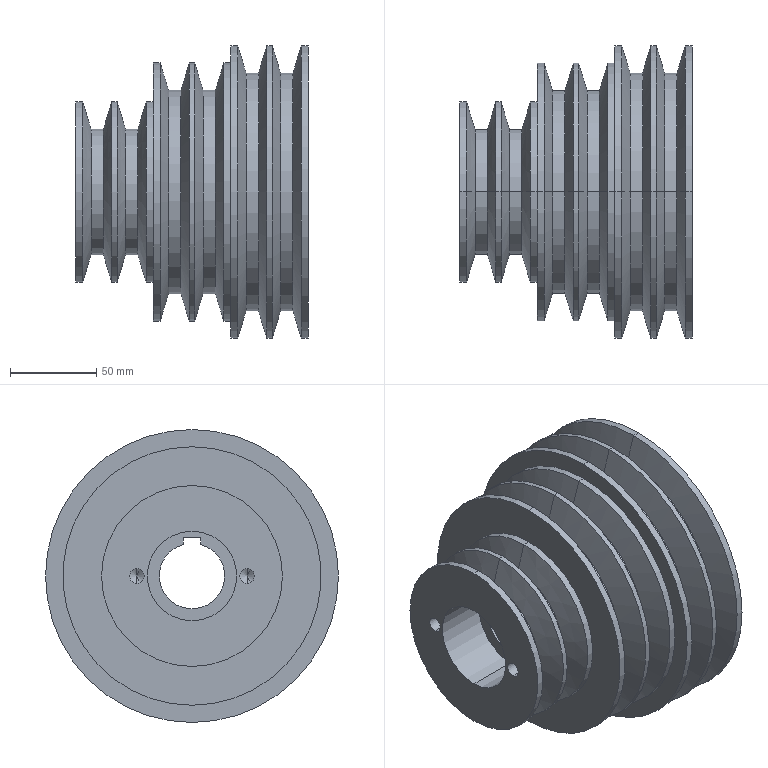Part | SolidWorks | features HoleWzd 1, ICE 1, Revolution 1 | 1 solid | 79 faces | box 135 x 170 x 170 mm | volume 1424823 mm3 | cylinder 41 | cone 28 | plane 10 | commonest cylinder face diameters 105 x6 150 x6 170 x6 8.5 x4 73 x4 118 x4